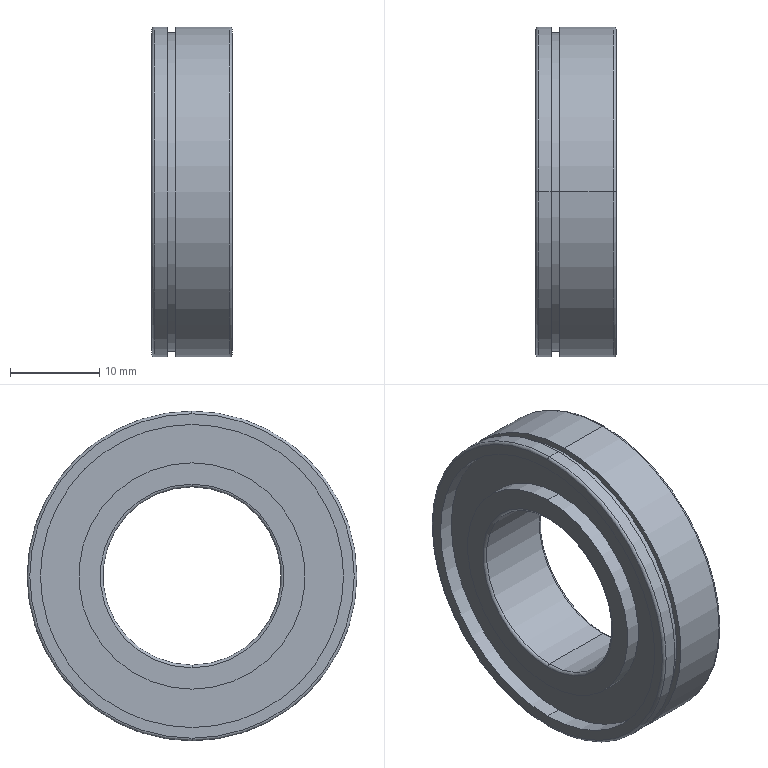Part | STEP file | SB6904ZZNR-Part-1-3 | 1 solid | 32 faces | box 9 x 37 x 37 mm | volume 5829 mm3 | cylinder 16 | torus 8 | plane 8 | commonest cylinder face diameters 25.4 x4 34 x4 37 x4 20 x2 35.7 x2
STEP:
#1=CARTESIAN_POINT('',(0.,0.,18.2));
#2=VERTEX_POINT('',#1);
#3=CARTESIAN_POINT('',(0.,0.,-18.2));
#4=VERTEX_POINT('',#3);
#5=CARTESIAN_POINT('',(0.,0.,0.));
#6=DIRECTION('',(-1.,0.,0.));
#7=DIRECTION('',(0.,0.,-1.));
#8=AXIS2_PLACEMENT_3D('',#5,#6,#7);
#9=CIRCLE('',#8,18.2);
#10=EDGE_CURVE('',#2,#4,#9,.T.);
#11=ORIENTED_EDGE('',*,*,#10,.F.);
#12=CARTESIAN_POINT('',(0.3,0.,18.5));
#13=VERTEX_POINT('',#12);
#14=CARTESIAN_POINT('',(0.3,0.,18.2));
#15=DIRECTION('',(0.,1.,0.));
#16=DIRECTION('',(0.,0.,1.));
#17=AXIS2_PLACEMENT_3D('',#14,#15,#16);
#18=CIRCLE('',#17,0.3);
#19=EDGE_CURVE('',#2,#13,#18,.T.);
#20=ORIENTED_EDGE('',*,*,#19,.T.);
#21=CARTESIAN_POINT('',(0.3,0.,-18.5));
#22=VERTEX_POINT('',#21);
#23=CARTESIAN_POINT('',(0.3,0.,0.));
#24=DIRECTION('',(1.,0.,0.));
#25=DIRECTION('',(0.,0.,-1.));
#26=AXIS2_PLACEMENT_3D('',#23,#24,#25);
#27=CIRCLE('',#26,18.5);
#28=EDGE_CURVE('',#22,#13,#27,.T.);
#29=ORIENTED_EDGE('',*,*,#28,.F.);
#30=CARTESIAN_POINT('',(0.3,0.,-18.2));
#31=DIRECTION('',(0.,-1.,0.));
#32=DIRECTION('',(0.,0.,-1.));
#33=AXIS2_PLACEMENT_3D('',#30,#31,#32);
#34=CIRCLE('',#33,0.3);
#35=EDGE_CURVE('',#4,#22,#34,.T.);
#36=ORIENTED_EDGE('',*,*,#35,.F.);
#37=EDGE_LOOP('',(#11,#20,#29,#36));
#38=FACE_OUTER_BOUND('',#37,.T.);
#39=CARTESIAN_POINT('',(0.3,0.,0.));
#40=DIRECTION('',(1.,0.,0.));
#41=DIRECTION('',(0.,0.,-1.));
#42=AXIS2_PLACEMENT_3D('',#39,#40,#41);
#43=TOROIDAL_SURFACE('',#42,18.2,0.3);
#44=ADVANCED_FACE('',(#38),#43,.T.);
#45=CARTESIAN_POINT('',(0.3,0.,10.));
#46=VERTEX_POINT('',#45);
#47=CARTESIAN_POINT('',(0.3,0.,-10.));
#48=VERTEX_POINT('',#47);
#49=CARTESIAN_POINT('',(0.3,0.,0.));
#50=DIRECTION('',(-1.,0.,0.));
#51=DIRECTION('',(0.,0.,-1.));
#52=AXIS2_PLACEMENT_3D('',#49,#50,#51);
#53=CIRCLE('',#52,10.);
#54=EDGE_CURVE('',#46,#48,#53,.T.);
#55=ORIENTED_EDGE('',*,*,#54,.F.);
#56=CARTESIAN_POINT('',(0.,0.,10.3));
#57=VERTEX_POINT('',#56);
#58=CARTESIAN_POINT('',(0.3,0.,10.3));
#59=DIRECTION('',(0.,1.,0.));
#60=DIRECTION('',(0.,0.,1.));
#61=AXIS2_PLACEMENT_3D('',#58,#59,#60);
#62=CIRCLE('',#61,0.3);
#63=EDGE_CURVE('',#46,#57,#62,.T.);
#64=ORIENTED_EDGE('',*,*,#63,.T.);
#65=CARTESIAN_POINT('',(0.,0.,-10.3));
#66=VERTEX_POINT('',#65);
#67=CARTESIAN_POINT('',(0.,0.,0.));
#68=DIRECTION('',(1.,0.,0.));
#69=DIRECTION('',(0.,0.,-1.));
#70=AXIS2_PLACEMENT_3D('',#67,#68,#69);
#71=CIRCLE('',#70,10.3);
#72=EDGE_CURVE('',#66,#57,#71,.T.);
#73=ORIENTED_EDGE('',*,*,#72,.F.);
#74=CARTESIAN_POINT('',(0.3,0.,-10.3));
#75=DIRECTION('',(0.,-1.,0.));
#76=DIRECTION('',(0.,0.,-1.));
#77=AXIS2_PLACEMENT_3D('',#74,#75,#76);
#78=CIRCLE('',#77,0.3);
#79=EDGE_CURVE('',#48,#66,#78,.T.);
#80=ORIENTED_EDGE('',*,*,#79,.F.);
#81=EDGE_LOOP('',(#55,#64,#73,#80));
#82=FACE_OUTER_BOUND('',#81,.T.);
#83=CARTESIAN_POINT('',(0.3,0.,0.));
#84=DIRECTION('',(1.,0.,0.));
#85=DIRECTION('',(0.,0.,-1.));
#86=AXIS2_PLACEMENT_3D('',#83,#84,#85);
#87=TOROIDAL_SURFACE('',#86,10.3,0.3);
#88=ADVANCED_FACE('',(#82),#87,.T.);
#89=CARTESIAN_POINT('',(8.7,0.,-10.));
#90=VERTEX_POINT('',#89);
#91=CARTESIAN_POINT('',(8.7,0.,10.));
#92=VERTEX_POINT('',#91);
#93=CARTESIAN_POINT('',(8.7,0.,0.));
#94=DIRECTION('',(1.,0.,0.));
#95=DIRECTION('',(0.,0.,1.));
#96=AXIS2_PLACEMENT_3D('',#93,#94,#95);
#97=CIRCLE('',#96,10.);
#98=EDGE_CURVE('',#90,#92,#97,.T.);
#99=ORIENTED_EDGE('',*,*,#98,.F.);
#100=CARTESIAN_POINT('',(9.,0.,-10.3));
#101=VERTEX_POINT('',#100);
#102=CARTESIAN_POINT('',(8.7,0.,-10.3));
#103=DIRECTION('',(0.,1.,0.));
#104=DIRECTION('',(0.,0.,1.));
#105=AXIS2_PLACEMENT_3D('',#102,#103,#104);
#106=CIRCLE('',#105,0.3);
#107=EDGE_CURVE('',#90,#101,#106,.T.);
#108=ORIENTED_EDGE('',*,*,#107,.T.);
#109=CARTESIAN_POINT('',(9.,0.,10.3));
#110=VERTEX_POINT('',#109);
#111=CARTESIAN_POINT('',(9.,0.,0.));
#112=DIRECTION('',(-1.,0.,0.));
#113=DIRECTION('',(0.,0.,1.));
#114=AXIS2_PLACEMENT_3D('',#111,#112,#113);
#115=CIRCLE('',#114,10.3);
#116=EDGE_CURVE('',#110,#101,#115,.T.);
#117=ORIENTED_EDGE('',*,*,#116,.F.);
#118=CARTESIAN_POINT('',(8.7,0.,10.3));
#119=DIRECTION('',(0.,-1.,0.));
#120=DIRECTION('',(0.,0.,-1.));
#121=AXIS2_PLACEMENT_3D('',#118,#119,#120);
#122=CIRCLE('',#121,0.3);
#123=EDGE_CURVE('',#92,#110,#122,.T.);
#124=ORIENTED_EDGE('',*,*,#123,.F.);
#125=EDGE_LOOP('',(#99,#108,#117,#124));
#126=FACE_OUTER_BOUND('',#125,.T.);
#127=CARTESIAN_POINT('',(8.7,0.,0.));
#128=DIRECTION('',(-1.,0.,0.));
#129=DIRECTION('',(0.,0.,1.));
#130=AXIS2_PLACEMENT_3D('',#127,#128,#129);
#131=TOROIDAL_SURFACE('',#130,10.3,0.3);
#132=ADVANCED_FACE('',(#126),#131,.T.);
#133=CARTESIAN_POINT('',(9.,0.,-18.2));
#134=VERTEX_POINT('',#133);
#135=CARTESIAN_POINT('',(9.,0.,18.2));
#136=VERTEX_POINT('',#135);
#137=CARTESIAN_POINT('',(9.,0.,0.));
#138=DIRECTION('',(1.,0.,0.));
#139=DIRECTION('',(0.,0.,1.));
#140=AXIS2_PLACEMENT_3D('',#137,#138,#139);
#141=CIRCLE('',#140,18.2);
#142=EDGE_CURVE('',#134,#136,#141,.T.);
#143=ORIENTED_EDGE('',*,*,#142,.F.);
#144=CARTESIAN_POINT('',(8.7,0.,-18.5));
#145=VERTEX_POINT('',#144);
#146=CARTESIAN_POINT('',(8.7,0.,-18.2));
#147=DIRECTION('',(0.,1.,0.));
#148=DIRECTION('',(0.,0.,1.));
#149=AXIS2_PLACEMENT_3D('',#146,#147,#148);
#150=CIRCLE('',#149,0.3);
#151=EDGE_CURVE('',#134,#145,#150,.T.);
#152=ORIENTED_EDGE('',*,*,#151,.T.);
#153=CARTESIAN_POINT('',(8.7,0.,18.5));
#154=VERTEX_POINT('',#153);
#155=CARTESIAN_POINT('',(8.7,0.,0.));
#156=DIRECTION('',(-1.,0.,0.));
#157=DIRECTION('',(0.,0.,1.));
#158=AXIS2_PLACEMENT_3D('',#155,#156,#157);
#159=CIRCLE('',#158,18.5);
#160=EDGE_CURVE('',#154,#145,#159,.T.);
#161=ORIENTED_EDGE('',*,*,#160,.F.);
#162=CARTESIAN_POINT('',(8.7,0.,18.2));
#163=DIRECTION('',(0.,-1.,0.));
#164=DIRECTION('',(0.,0.,-1.));
#165=AXIS2_PLACEMENT_3D('',#162,#163,#164);
#166=CIRCLE('',#165,0.3);
#167=EDGE_CURVE('',#136,#154,#166,.T.);
#168=ORIENTED_EDGE('',*,*,#167,.F.);
#169=EDGE_LOOP('',(#143,#152,#161,#168));
#170=FACE_OUTER_BOUND('',#169,.T.);
#171=CARTESIAN_POINT('',(8.7,0.,0.));
#172=DIRECTION('',(-1.,0.,0.));
#173=DIRECTION('',(0.,0.,1.));
#174=AXIS2_PLACEMENT_3D('',#171,#172,#173);
#175=TOROIDAL_SURFACE('',#174,18.2,0.3);
#176=ADVANCED_FACE('',(#170),#175,.T.);
#177=CARTESIAN_POINT('',(1.7,0.,-17.));
#178=VERTEX_POINT('',#177);
#179=CARTESIAN_POINT('',(1.7,0.,17.));
#180=VERTEX_POINT('',#179);
#181=CARTESIAN_POINT('',(1.7,0.,0.));
#182=DIRECTION('',(-1.,0.,0.));
#183=DIRECTION('',(0.,0.,1.));
#184=AXIS2_PLACEMENT_3D('',#181,#182,#183);
#185=CIRCLE('',#184,17.);
#186=EDGE_CURVE('',#178,#180,#185,.T.);
#187=ORIENTED_EDGE('',*,*,#186,.F.);
#188=CARTESIAN_POINT('',(0.,0.,-17.));
#189=VERTEX_POINT('',#188);
#190=CARTESIAN_POINT('',(0.,0.,-17.));
#191=DIRECTION('',(-1.,0.,0.));
#192=VECTOR('',#191,1000.);
#193=LINE('',#190,#192);
#194=EDGE_CURVE('',#178,#189,#193,.T.);
#195=ORIENTED_EDGE('',*,*,#194,.T.);
#196=CARTESIAN_POINT('',(0.,0.,17.));
#197=VERTEX_POINT('',#196);
#198=CARTESIAN_POINT('',(0.,0.,0.));
#199=DIRECTION('',(-1.,0.,0.));
#200=DIRECTION('',(0.,0.,1.));
#201=AXIS2_PLACEMENT_3D('',#198,#199,#200);
#202=CIRCLE('',#201,17.);
#203=EDGE_CURVE('',#189,#197,#202,.T.);
#204=ORIENTED_EDGE('',*,*,#203,.T.);
#205=CARTESIAN_POINT('',(0.,0.,17.));
#206=DIRECTION('',(-1.,0.,0.));
#207=VECTOR('',#206,1000.);
#208=LINE('',#205,#207);
#209=EDGE_CURVE('',#180,#197,#208,.T.);
#210=ORIENTED_EDGE('',*,*,#209,.F.);
#211=EDGE_LOOP('',(#187,#195,#204,#210));
#212=FACE_OUTER_BOUND('',#211,.T.);
#213=CARTESIAN_POINT('',(0.,0.,0.));
#214=DIRECTION('',(-1.,0.,0.));
#215=DIRECTION('',(0.,0.,1.));
#216=AXIS2_PLACEMENT_3D('',#213,#214,#215);
#217=CYLINDRICAL_SURFACE('',#216,17.);
#218=ADVANCED_FACE('',(#212),#217,.F.);
#219=CARTESIAN_POINT('',(1.7,0.,12.7));
#220=VERTEX_POINT('',#219);
#221=CARTESIAN_POINT('',(1.7,0.,-12.7));
#222=VERTEX_POINT('',#221);
#223=CARTESIAN_POINT('',(1.7,0.,0.));
#224=DIRECTION('',(-1.,0.,0.));
#225=DIRECTION('',(0.,0.,1.));
#226=AXIS2_PLACEMENT_3D('',#223,#224,#225);
#227=CIRCLE('',#226,12.7);
#228=EDGE_CURVE('',#220,#222,#227,.T.);
#229=ORIENTED_EDGE('',*,*,#228,.T.);
#230=CARTESIAN_POINT('',(0.,0.,-12.7));
#231=VERTEX_POINT('',#230);
#232=CARTESIAN_POINT('',(0.,0.,-12.7));
#233=DIRECTION('',(-1.,0.,0.));
#234=VECTOR('',#233,1000.);
#235=LINE('',#232,#234);
#236=EDGE_CURVE('',#222,#231,#235,.T.);
#237=ORIENTED_EDGE('',*,*,#236,.T.);
#238=CARTESIAN_POINT('',(0.,0.,12.7));
#239=VERTEX_POINT('',#238);
#240=CARTESIAN_POINT('',(0.,0.,0.));
#241=DIRECTION('',(-1.,0.,0.));
#242=DIRECTION('',(0.,0.,1.));
#243=AXIS2_PLACEMENT_3D('',#240,#241,#242);
#244=CIRCLE('',#243,12.7);
#245=EDGE_CURVE('',#239,#231,#244,.T.);
#246=ORIENTED_EDGE('',*,*,#245,.F.);
#247=CARTESIAN_POINT('',(0.,0.,12.7));
#248=DIRECTION('',(-1.,0.,0.));
#249=VECTOR('',#248,1000.);
#250=LINE('',#247,#249);
#251=EDGE_CURVE('',#220,#239,#250,.T.);
#252=ORIENTED_EDGE('',*,*,#251,.F.);
#253=EDGE_LOOP('',(#229,#237,#246,#252));
#254=FACE_OUTER_BOUND('',#253,.T.);
#255=CARTESIAN_POINT('',(0.,0.,0.));
#256=DIRECTION('',(-1.,0.,0.));
#257=DIRECTION('',(0.,0.,1.));
#258=AXIS2_PLACEMENT_3D('',#255,#256,#257);
#259=CYLINDRICAL_SURFACE('',#258,12.7);
#260=ADVANCED_FACE('',(#254),#259,.T.);
#261=CARTESIAN_POINT('',(8.7,0.,0.));
#262=DIRECTION('',(1.,0.,0.));
#263=DIRECTION('',(0.,0.,1.));
#264=AXIS2_PLACEMENT_3D('',#261,#262,#263);
#265=CIRCLE('',#264,10.);
#266=EDGE_CURVE('',#92,#90,#265,.T.);
#267=ORIENTED_EDGE('',*,*,#266,.T.);
#268=CARTESIAN_POINT('',(0.,0.,-10.));
#269=DIRECTION('',(-1.,0.,0.));
#270=VECTOR('',#269,1000.);
#271=LINE('',#268,#270);
#272=EDGE_CURVE('',#90,#48,#271,.T.);
#273=ORIENTED_EDGE('',*,*,#272,.T.);
#274=CARTESIAN_POINT('',(0.3,0.,0.));
#275=DIRECTION('',(-1.,0.,0.));
#276=DIRECTION('',(0.,0.,-1.));
#277=AXIS2_PLACEMENT_3D('',#274,#275,#276);
#278=CIRCLE('',#277,10.);
#279=EDGE_CURVE('',#48,#46,#278,.T.);
#280=ORIENTED_EDGE('',*,*,#279,.T.);
#281=CARTESIAN_POINT('',(0.,0.,10.));
#282=DIRECTION('',(-1.,0.,0.));
#283=VECTOR('',#282,1000.);
#284=LINE('',#281,#283);
#285=EDGE_CURVE('',#92,#46,#284,.T.);
#286=ORIENTED_EDGE('',*,*,#285,.F.);
#287=EDGE_LOOP('',(#267,#273,#280,#286));
#288=FACE_OUTER_BOUND('',#287,.T.);
#289=CARTESIAN_POINT('',(0.,0.,0.));
#290=DIRECTION('',(-1.,0.,0.));
#291=DIRECTION('',(0.,0.,1.));
#292=AXIS2_PLACEMENT_3D('',#289,#290,#291);
#293=CYLINDRICAL_SURFACE('',#292,10.);
#294=ADVANCED_FACE('',(#288),#293,.F.);
#295=CARTESIAN_POINT('',(9.,0.,12.7));
#296=VERTEX_POINT('',#295);
#297=CARTESIAN_POINT('',(9.,0.,-12.7));
#298=VERTEX_POINT('',#297);
#299=CARTESIAN_POINT('',(9.,0.,0.));
#300=DIRECTION('',(-1.,0.,0.));
#301=DIRECTION('',(0.,0.,1.));
#302=AXIS2_PLACEMENT_3D('',#299,#300,#301);
#303=CIRCLE('',#302,12.7);
#304=EDGE_CURVE('',#296,#298,#303,.T.);
#305=ORIENTED_EDGE('',*,*,#304,.T.);
#306=CARTESIAN_POINT('',(8.35,0.,-12.7));
#307=VERTEX_POINT('',#306);
#308=CARTESIAN_POINT('',(0.,0.,-12.7));
#309=DIRECTION('',(-1.,0.,0.));
#310=VECTOR('',#309,1000.);
#311=LINE('',#308,#310);
#312=EDGE_CURVE('',#298,#307,#311,.T.);
#313=ORIENTED_EDGE('',*,*,#312,.T.);
#314=CARTESIAN_POINT('',(8.35,0.,12.7));
#315=VERTEX_POINT('',#314);
#316=CARTESIAN_POINT('',(8.35,0.,0.));
#317=DIRECTION('',(-1.,0.,0.));
#318=DIRECTION('',(0.,0.,1.));
#319=AXIS2_PLACEMENT_3D('',#316,#317,#318);
#320=CIRCLE('',#319,12.7);
#321=EDGE_CURVE('',#315,#307,#320,.T.);
#322=ORIENTED_EDGE('',*,*,#321,.F.);
#323=CARTESIAN_POINT('',(0.,0.,12.7));
#324=DIRECTION('',(-1.,0.,0.));
#325=VECTOR('',#324,1000.);
#326=LINE('',#323,#325);
#327=EDGE_CURVE('',#296,#315,#326,.T.);
#328=ORIENTED_EDGE('',*,*,#327,.F.);
#329=EDGE_LOOP('',(#305,#313,#322,#328));
#330=FACE_OUTER_BOUND('',#329,.T.);
#331=CARTESIAN_POINT('',(0.,0.,0.));
#332=DIRECTION('',(-1.,0.,0.));
#333=DIRECTION('',(0.,0.,1.));
#334=AXIS2_PLACEMENT_3D('',#331,#332,#333);
#335=CYLINDRICAL_SURFACE('',#334,12.7);
#336=ADVANCED_FACE('',(#330),#335,.T.);
#337=CARTESIAN_POINT('',(9.,0.,-17.));
#338=VERTEX_POINT('',#337);
#339=CARTESIAN_POINT('',(9.,0.,17.));
#340=VERTEX_POINT('',#339);
#341=CARTESIAN_POINT('',(9.,0.,0.));
#342=DIRECTION('',(-1.,0.,0.));
#343=DIRECTION('',(0.,0.,1.));
#344=AXIS2_PLACEMENT_3D('',#341,#342,#343);
#345=CIRCLE('',#344,17.);
#346=EDGE_CURVE('',#338,#340,#345,.T.);
#347=ORIENTED_EDGE('',*,*,#346,.F.);
#348=CARTESIAN_POINT('',(8.35,0.,-17.));
#349=VERTEX_POINT('',#348);
#350=CARTESIAN_POINT('',(0.,0.,-17.));
#351=DIRECTION('',(-1.,0.,0.));
#352=VECTOR('',#351,1000.);
#353=LINE('',#350,#352);
#354=EDGE_CURVE('',#338,#349,#353,.T.);
#355=ORIENTED_EDGE('',*,*,#354,.T.);
#356=CARTESIAN_POINT('',(8.35,0.,17.));
#357=VERTEX_POINT('',#356);
#358=CARTESIAN_POINT('',(8.35,0.,0.));
#359=DIRECTION('',(-1.,0.,0.));
#360=DIRECTION('',(0.,0.,1.));
#361=AXIS2_PLACEMENT_3D('',#358,#359,#360);
#362=CIRCLE('',#361,17.);
#363=EDGE_CURVE('',#349,#357,#362,.T.);
#364=ORIENTED_EDGE('',*,*,#363,.T.);
#365=CARTESIAN_POINT('',(0.,0.,17.));
#366=DIRECTION('',(-1.,0.,0.));
#367=VECTOR('',#366,1000.);
#368=LINE('',#365,#367);
#369=EDGE_CURVE('',#340,#357,#368,.T.);
#370=ORIENTED_EDGE('',*,*,#369,.F.);
#371=EDGE_LOOP('',(#347,#355,#364,#370));
#372=FACE_OUTER_BOUND('',#371,.T.);
#373=CARTESIAN_POINT('',(0.,0.,0.));
#374=DIRECTION('',(-1.,0.,0.));
#375=DIRECTION('',(0.,0.,1.));
#376=AXIS2_PLACEMENT_3D('',#373,#374,#375);
#377=CYLINDRICAL_SURFACE('',#376,17.);
#378=ADVANCED_FACE('',(#372),#377,.F.);
#379=ORIENTED_EDGE('',*,*,#160,.T.);
#380=CARTESIAN_POINT('',(2.65,0.,-18.5));
#381=VERTEX_POINT('',#380);
#382=CARTESIAN_POINT('',(0.,0.,-18.5));
#383=DIRECTION('',(-1.,0.,0.));
#384=VECTOR('',#383,1000.);
#385=LINE('',#382,#384);
#386=EDGE_CURVE('',#145,#381,#385,.T.);
#387=ORIENTED_EDGE('',*,*,#386,.T.);
#388=CARTESIAN_POINT('',(2.65,0.,18.5));
#389=VERTEX_POINT('',#388);
#390=CARTESIAN_POINT('',(2.65,0.,0.));
#391=DIRECTION('',(-1.,0.,0.));
#392=DIRECTION('',(0.,0.,1.));
#393=AXIS2_PLACEMENT_3D('',#390,#391,#392);
#394=CIRCLE('',#393,18.5);
#395=EDGE_CURVE('',#389,#381,#394,.T.);
#396=ORIENTED_EDGE('',*,*,#395,.F.);
#397=CARTESIAN_POINT('',(0.,0.,18.5));
#398=DIRECTION('',(-1.,0.,0.));
#399=VECTOR('',#398,1000.);
#400=LINE('',#397,#399);
#401=EDGE_CURVE('',#154,#389,#400,.T.);
#402=ORIENTED_EDGE('',*,*,#401,.F.);
#403=EDGE_LOOP('',(#379,#387,#396,#402));
#404=FACE_OUTER_BOUND('',#403,.T.);
#405=CARTESIAN_POINT('',(0.,0.,0.));
#406=DIRECTION('',(-1.,0.,0.));
#407=DIRECTION('',(0.,0.,1.));
#408=AXIS2_PLACEMENT_3D('',#405,#406,#407);
#409=CYLINDRICAL_SURFACE('',#408,18.5);
#410=ADVANCED_FACE('',(#404),#409,.T.);
#411=CARTESIAN_POINT('',(2.65,0.,17.85));
#412=VERTEX_POINT('',#411);
#413=CARTESIAN_POINT('',(2.65,0.,-17.85));
#414=VERTEX_POINT('',#413);
#415=CARTESIAN_POINT('',(2.65,0.,0.));
#416=DIRECTION('',(-1.,0.,0.));
#417=DIRECTION('',(0.,0.,1.));
#418=AXIS2_PLACEMENT_3D('',#415,#416,#417);
#419=CIRCLE('',#418,17.85);
#420=EDGE_CURVE('',#412,#414,#419,.T.);
#421=ORIENTED_EDGE('',*,*,#420,.T.);
#422=CARTESIAN_POINT('',(1.7,0.,-17.85));
#423=VERTEX_POINT('',#422);
#424=CARTESIAN_POINT('',(1.05,0.,-17.85));
#425=DIRECTION('',(-1.,0.,0.));
#426=VECTOR('',#425,1000.);
#427=LINE('',#424,#426);
#428=EDGE_CURVE('',#414,#423,#427,.T.);
#429=ORIENTED_EDGE('',*,*,#428,.T.);
#430=CARTESIAN_POINT('',(1.7,0.,17.85));
#431=VERTEX_POINT('',#430);
#432=CARTESIAN_POINT('',(1.7,0.,0.));
#433=DIRECTION('',(-1.,0.,0.));
#434=DIRECTION('',(0.,0.,1.));
#435=AXIS2_PLACEMENT_3D('',#432,#433,#434);
#436=CIRCLE('',#435,17.85);
#437=EDGE_CURVE('',#431,#423,#436,.T.);
#438=ORIENTED_EDGE('',*,*,#437,.F.);
#439=CARTESIAN_POINT('',(1.05,0.,17.85));
#440=DIRECTION('',(-1.,0.,0.));
#441=VECTOR('',#440,1000.);
#442=LINE('',#439,#441);
#443=EDGE_CURVE('',#412,#431,#442,.T.);
#444=ORIENTED_EDGE('',*,*,#443,.F.);
#445=EDGE_LOOP('',(#421,#429,#438,#444));
#446=FACE_OUTER_BOUND('',#445,.T.);
#447=CARTESIAN_POINT('',(1.05,0.,0.));
#448=DIRECTION('',(-1.,0.,0.));
#449=DIRECTION('',(0.,0.,1.));
#450=AXIS2_PLACEMENT_3D('',#447,#448,#449);
#451=CYLINDRICAL_SURFACE('',#450,17.85);
#452=ADVANCED_FACE('',(#446),#451,.T.);
#453=CARTESIAN_POINT('',(1.7,0.,18.5));
#454=VERTEX_POINT('',#453);
#455=CARTESIAN_POINT('',(1.7,0.,-18.5));
#456=VERTEX_POINT('',#455);
#457=CARTESIAN_POINT('',(1.7,0.,0.));
#458=DIRECTION('',(-1.,0.,0.));
#459=DIRECTION('',(0.,0.,1.));
#460=AXIS2_PLACEMENT_3D('',#457,#458,#459);
#461=CIRCLE('',#460,18.5);
#462=EDGE_CURVE('',#454,#456,#461,.T.);
#463=ORIENTED_EDGE('',*,*,#462,.T.);
#464=CARTESIAN_POINT('',(0.,0.,-18.5));
#465=DIRECTION('',(-1.,0.,0.));
#466=VECTOR('',#465,1000.);
#467=LINE('',#464,#466);
#468=EDGE_CURVE('',#456,#22,#467,.T.);
#469=ORIENTED_EDGE('',*,*,#468,.T.);
#470=ORIENTED_EDGE('',*,*,#28,.T.);
#471=CARTESIAN_POINT('',(0.,0.,18.5));
#472=DIRECTION('',(-1.,0.,0.));
#473=VECTOR('',#472,1000.);
#474=LINE('',#471,#473);
#475=EDGE_CURVE('',#454,#13,#474,.T.);
#476=ORIENTED_EDGE('',*,*,#475,.F.);
#477=EDGE_LOOP('',(#463,#469,#470,#476));
#478=FACE_OUTER_BOUND('',#477,.T.);
#479=CARTESIAN_POINT('',(0.,0.,0.));
#480=DIRECTION('',(-1.,0.,0.));
#481=DIRECTION('',(0.,0.,1.));
#482=AXIS2_PLACEMENT_3D('',#479,#480,#481);
#483=CYLINDRICAL_SURFACE('',#482,18.5);
#484=ADVANCED_FACE('',(#478),#483,.T.);
#485=CARTESIAN_POINT('',(0.,0.,0.));
#486=DIRECTION('',(-1.,0.,0.));
#487=DIRECTION('',(0.,0.,-1.));
#488=AXIS2_PLACEMENT_3D('',#485,#486,#487);
#489=CIRCLE('',#488,18.2);
#490=EDGE_CURVE('',#4,#2,#489,.T.);
#491=ORIENTED_EDGE('',*,*,#490,.T.);
#492=ORIENTED_EDGE('',*,*,#10,.T.);
#493=EDGE_LOOP('',(#491,#492));
#494=FACE_OUTER_BOUND('',#493,.T.);
#495=CARTESIAN_POINT('',(0.,0.,0.));
#496=DIRECTION('',(-1.,0.,0.));
#497=DIRECTION('',(0.,0.,1.));
#498=AXIS2_PLACEMENT_3D('',#495,#496,#497);
#499=CIRCLE('',#498,17.);
#500=EDGE_CURVE('',#197,#189,#499,.T.);
#501=ORIENTED_EDGE('',*,*,#500,.F.);
#502=ORIENTED_EDGE('',*,*,#203,.F.);
#503=EDGE_LOOP('',(#501,#502));
#504=FACE_BOUND('',#503,.T.);
#505=CARTESIAN_POINT('',(0.,17.,0.));
#506=DIRECTION('',(1.,0.,0.));
#507=DIRECTION('',(0.,0.,-1.));
#508=AXIS2_PLACEMENT_3D('',#505,#506,#507);
#509=PLANE('',#508);
#510=ADVANCED_FACE('',(#494,#504),#509,.F.);
#511=ORIENTED_EDGE('',*,*,#468,.F.);
#512=CARTESIAN_POINT('',(1.7,0.,0.));
#513=DIRECTION('',(-1.,0.,0.));
#514=DIRECTION('',(0.,0.,1.));
#515=AXIS2_PLACEMENT_3D('',#512,#513,#514);
#516=CIRCLE('',#515,18.5);
#517=EDGE_CURVE('',#456,#454,#516,.T.);
#518=ORIENTED_EDGE('',*,*,#517,.T.);
#519=ORIENTED_EDGE('',*,*,#475,.T.);
#520=CARTESIAN_POINT('',(0.3,0.,0.));
#521=DIRECTION('',(1.,0.,0.));
#522=DIRECTION('',(0.,0.,-1.));
#523=AXIS2_PLACEMENT_3D('',#520,#521,#522);
#524=CIRCLE('',#523,18.5);
#525=EDGE_CURVE('',#13,#22,#524,.T.);
#526=ORIENTED_EDGE('',*,*,#525,.T.);
#527=EDGE_LOOP('',(#511,#518,#519,#526));
#528=FACE_OUTER_BOUND('',#527,.T.);
#529=CARTESIAN_POINT('',(0.,0.,0.));
#530=DIRECTION('',(-1.,0.,0.));
#531=DIRECTION('',(0.,0.,1.));
#532=AXIS2_PLACEMENT_3D('',#529,#530,#531);
#533=CYLINDRICAL_SURFACE('',#532,18.5);
#534=ADVANCED_FACE('',(#528),#533,.T.);
#535=ORIENTED_EDGE('',*,*,#462,.F.);
#536=ORIENTED_EDGE('',*,*,#517,.F.);
#537=EDGE_LOOP('',(#535,#536));
#538=FACE_OUTER_BOUND('',#537,.T.);
#539=ORIENTED_EDGE('',*,*,#437,.T.);
#540=CARTESIAN_POINT('',(1.7,0.,0.));
#541=DIRECTION('',(-1.,0.,0.));
#542=DIRECTION('',(0.,0.,1.));
#543=AXIS2_PLACEMENT_3D('',#540,#541,#542);
#544=CIRCLE('',#543,17.85);
#545=EDGE_CURVE('',#423,#431,#544,.T.);
#546=ORIENTED_EDGE('',*,*,#545,.T.);
#547=EDGE_LOOP('',(#539,#546));
#548=FACE_BOUND('',#547,.T.);
#549=CARTESIAN_POINT('',(1.7,18.5,0.));
#550=DIRECTION('',(-1.,0.,0.));
#551=DIRECTION('',(0.,0.,1.));
#552=AXIS2_PLACEMENT_3D('',#549,#550,#551);
#553=PLANE('',#552);
#554=ADVANCED_FACE('',(#538,#548),#553,.F.);
#555=ORIENTED_EDGE('',*,*,#428,.F.);
#556=CARTESIAN_POINT('',(2.65,0.,0.));
#557=DIRECTION('',(-1.,0.,0.));
#558=DIRECTION('',(0.,0.,1.));
#559=AXIS2_PLACEMENT_3D('',#556,#557,#558);
#560=CIRCLE('',#559,17.85);
#561=EDGE_CURVE('',#414,#412,#560,.T.);
#562=ORIENTED_EDGE('',*,*,#561,.T.);
#563=ORIENTED_EDGE('',*,*,#443,.T.);
#564=ORIENTED_EDGE('',*,*,#545,.F.);
#565=EDGE_LOOP('',(#555,#562,#563,#564));
#566=FACE_OUTER_BOUND('',#565,.T.);
#567=CARTESIAN_POINT('',(1.05,0.,0.));
#568=DIRECTION('',(-1.,0.,0.));
#569=DIRECTION('',(0.,0.,1.));
#570=AXIS2_PLACEMENT_3D('',#567,#568,#569);
#571=CYLINDRICAL_SURFACE('',#570,17.85);
#572=ADVANCED_FACE('',(#566),#571,.T.);
#573=ORIENTED_EDGE('',*,*,#420,.F.);
#574=ORIENTED_EDGE('',*,*,#561,.F.);
#575=EDGE_LOOP('',(#573,#574));
#576=FACE_BOUND('',#575,.T.);
#577=ORIENTED_EDGE('',*,*,#395,.T.);
#578=CARTESIAN_POINT('',(2.65,0.,0.));
#579=DIRECTION('',(-1.,0.,0.));
#580=DIRECTION('',(0.,0.,1.));
#581=AXIS2_PLACEMENT_3D('',#578,#579,#580);
#582=CIRCLE('',#581,18.5);
#583=EDGE_CURVE('',#381,#389,#582,.T.);
#584=ORIENTED_EDGE('',*,*,#583,.T.);
#585=EDGE_LOOP('',(#577,#584));
#586=FACE_OUTER_BOUND('',#585,.T.);
#587=CARTESIAN_POINT('',(2.65,17.85,0.));
#588=DIRECTION('',(1.,0.,0.));
#589=DIRECTION('',(0.,0.,-1.));
#590=AXIS2_PLACEMENT_3D('',#587,#588,#589);
#591=PLANE('',#590);
#592=ADVANCED_FACE('',(#576,#586),#591,.F.);
#593=ORIENTED_EDGE('',*,*,#386,.F.);
#594=CARTESIAN_POINT('',(8.7,0.,0.));
#595=DIRECTION('',(-1.,0.,0.));
#596=DIRECTION('',(0.,0.,1.));
#597=AXIS2_PLACEMENT_3D('',#594,#595,#596);
#598=CIRCLE('',#597,18.5);
#599=EDGE_CURVE('',#145,#154,#598,.T.);
#600=ORIENTED_EDGE('',*,*,#599,.T.);
#601=ORIENTED_EDGE('',*,*,#401,.T.);
#602=ORIENTED_EDGE('',*,*,#583,.F.);
#603=EDGE_LOOP('',(#593,#600,#601,#602));
#604=FACE_OUTER_BOUND('',#603,.T.);
#605=CARTESIAN_POINT('',(0.,0.,0.));
#606=DIRECTION('',(-1.,0.,0.));
#607=DIRECTION('',(0.,0.,1.));
#608=AXIS2_PLACEMENT_3D('',#605,#606,#607);
#609=CYLINDRICAL_SURFACE('',#608,18.5);
#610=ADVANCED_FACE('',(#604),#609,.T.);
#611=CARTESIAN_POINT('',(9.,0.,0.));
#612=DIRECTION('',(1.,0.,0.));
#613=DIRECTION('',(0.,0.,1.));
#614=AXIS2_PLACEMENT_3D('',#611,#612,#613);
#615=CIRCLE('',#614,18.2);
#616=EDGE_CURVE('',#136,#134,#615,.T.);
#617=ORIENTED_EDGE('',*,*,#616,.T.);
#618=ORIENTED_EDGE('',*,*,#142,.T.);
#619=EDGE_LOOP('',(#617,#618));
#620=FACE_OUTER_BOUND('',#619,.T.);
#621=CARTESIAN_POINT('',(9.,0.,0.));
#622=DIRECTION('',(-1.,0.,0.));
#623=DIRECTION('',(0.,0.,1.));
#624=AXIS2_PLACEMENT_3D('',#621,#622,#623);
#625=CIRCLE('',#624,17.);
#626=EDGE_CURVE('',#340,#338,#625,.T.);
#627=ORIENTED_EDGE('',*,*,#626,.T.);
#628=ORIENTED_EDGE('',*,*,#346,.T.);
#629=EDGE_LOOP('',(#627,#628));
#630=FACE_BOUND('',#629,.T.);
#631=CARTESIAN_POINT('',(9.,18.5,0.));
#632=DIRECTION('',(-1.,0.,0.));
#633=DIRECTION('',(0.,0.,1.));
#634=AXIS2_PLACEMENT_3D('',#631,#632,#633);
#635=PLANE('',#634);
#636=ADVANCED_FACE('',(#620,#630),#635,.F.);
#637=ORIENTED_EDGE('',*,*,#354,.F.);
#638=ORIENTED_EDGE('',*,*,#626,.F.);
#639=ORIENTED_EDGE('',*,*,#369,.T.);
#640=CARTESIAN_POINT('',(8.35,0.,0.));
#641=DIRECTION('',(-1.,0.,0.));
#642=DIRECTION('',(0.,0.,1.));
#643=AXIS2_PLACEMENT_3D('',#640,#641,#642);
#644=CIRCLE('',#643,17.);
#645=EDGE_CURVE('',#357,#349,#644,.T.);
#646=ORIENTED_EDGE('',*,*,#645,.T.);
#647=EDGE_LOOP('',(#637,#638,#639,#646));
#648=FACE_OUTER_BOUND('',#647,.T.);
#649=CARTESIAN_POINT('',(0.,0.,0.));
#650=DIRECTION('',(-1.,0.,0.));
#651=DIRECTION('',(0.,0.,1.));
#652=AXIS2_PLACEMENT_3D('',#649,#650,#651);
#653=CYLINDRICAL_SURFACE('',#652,17.);
#654=ADVANCED_FACE('',(#648),#653,.F.);
#655=ORIENTED_EDGE('',*,*,#645,.F.);
#656=ORIENTED_EDGE('',*,*,#363,.F.);
#657=EDGE_LOOP('',(#655,#656));
#658=FACE_OUTER_BOUND('',#657,.T.);
#659=ORIENTED_EDGE('',*,*,#321,.T.);
#660=CARTESIAN_POINT('',(8.35,0.,0.));
#661=DIRECTION('',(-1.,0.,0.));
#662=DIRECTION('',(0.,0.,1.));
#663=AXIS2_PLACEMENT_3D('',#660,#661,#662);
#664=CIRCLE('',#663,12.7);
#665=EDGE_CURVE('',#307,#315,#664,.T.);
#666=ORIENTED_EDGE('',*,*,#665,.T.);
#667=EDGE_LOOP('',(#659,#666));
#668=FACE_BOUND('',#667,.T.);
#669=CARTESIAN_POINT('',(8.35,17.,0.));
#670=DIRECTION('',(-1.,0.,0.));
#671=DIRECTION('',(0.,0.,1.));
#672=AXIS2_PLACEMENT_3D('',#669,#670,#671);
#673=PLANE('',#672);
#674=ADVANCED_FACE('',(#658,#668),#673,.F.);
#675=ORIENTED_EDGE('',*,*,#312,.F.);
#676=CARTESIAN_POINT('',(9.,0.,0.));
#677=DIRECTION('',(-1.,0.,0.));
#678=DIRECTION('',(0.,0.,1.));
#679=AXIS2_PLACEMENT_3D('',#676,#677,#678);
#680=CIRCLE('',#679,12.7);
#681=EDGE_CURVE('',#298,#296,#680,.T.);
#682=ORIENTED_EDGE('',*,*,#681,.T.);
#683=ORIENTED_EDGE('',*,*,#327,.T.);
#684=ORIENTED_EDGE('',*,*,#665,.F.);
#685=EDGE_LOOP('',(#675,#682,#683,#684));
#686=FACE_OUTER_BOUND('',#685,.T.);
#687=CARTESIAN_POINT('',(0.,0.,0.));
#688=DIRECTION('',(-1.,0.,0.));
#689=DIRECTION('',(0.,0.,1.));
#690=AXIS2_PLACEMENT_3D('',#687,#688,#689);
#691=CYLINDRICAL_SURFACE('',#690,12.7);
#692=ADVANCED_FACE('',(#686),#691,.T.);
#693=ORIENTED_EDGE('',*,*,#116,.T.);
#694=CARTESIAN_POINT('',(9.,0.,0.));
#695=DIRECTION('',(-1.,0.,0.));
#696=DIRECTION('',(0.,0.,1.));
#697=AXIS2_PLACEMENT_3D('',#694,#695,#696);
#698=CIRCLE('',#697,10.3);
#699=EDGE_CURVE('',#101,#110,#698,.T.);
#700=ORIENTED_EDGE('',*,*,#699,.T.);
#701=EDGE_LOOP('',(#693,#700));
#702=FACE_BOUND('',#701,.T.);
#703=ORIENTED_EDGE('',*,*,#304,.F.);
#704=ORIENTED_EDGE('',*,*,#681,.F.);
#705=EDGE_LOOP('',(#703,#704));
#706=FACE_OUTER_BOUND('',#705,.T.);
#707=CARTESIAN_POINT('',(9.,12.7,0.));
#708=DIRECTION('',(-1.,0.,0.));
#709=DIRECTION('',(0.,0.,1.));
#710=AXIS2_PLACEMENT_3D('',#707,#708,#709);
#711=PLANE('',#710);
#712=ADVANCED_FACE('',(#702,#706),#711,.F.);
#713=ORIENTED_EDGE('',*,*,#272,.F.);
#714=ORIENTED_EDGE('',*,*,#98,.T.);
#715=ORIENTED_EDGE('',*,*,#285,.T.);
#716=ORIENTED_EDGE('',*,*,#54,.T.);
#717=EDGE_LOOP('',(#713,#714,#715,#716));
#718=FACE_OUTER_BOUND('',#717,.T.);
#719=CARTESIAN_POINT('',(0.,0.,0.));
#720=DIRECTION('',(-1.,0.,0.));
#721=DIRECTION('',(0.,0.,1.));
#722=AXIS2_PLACEMENT_3D('',#719,#720,#721);
#723=CYLINDRICAL_SURFACE('',#722,10.);
#724=ADVANCED_FACE('',(#718),#723,.F.);
#725=ORIENTED_EDGE('',*,*,#72,.T.);
#726=CARTESIAN_POINT('',(0.,0.,0.));
#727=DIRECTION('',(1.,0.,0.));
#728=DIRECTION('',(0.,0.,-1.));
#729=AXIS2_PLACEMENT_3D('',#726,#727,#728);
#730=CIRCLE('',#729,10.3);
#731=EDGE_CURVE('',#57,#66,#730,.T.);
#732=ORIENTED_EDGE('',*,*,#731,.T.);
#733=EDGE_LOOP('',(#725,#732));
#734=FACE_BOUND('',#733,.T.);
#735=ORIENTED_EDGE('',*,*,#245,.T.);
#736=CARTESIAN_POINT('',(0.,0.,0.));
#737=DIRECTION('',(-1.,0.,0.));
#738=DIRECTION('',(0.,0.,1.));
#739=AXIS2_PLACEMENT_3D('',#736,#737,#738);
#740=CIRCLE('',#739,12.7);
#741=EDGE_CURVE('',#231,#239,#740,.T.);
#742=ORIENTED_EDGE('',*,*,#741,.T.);
#743=EDGE_LOOP('',(#735,#742));
#744=FACE_OUTER_BOUND('',#743,.T.);
#745=CARTESIAN_POINT('',(0.,10.,0.));
#746=DIRECTION('',(1.,0.,0.));
#747=DIRECTION('',(0.,0.,-1.));
#748=AXIS2_PLACEMENT_3D('',#745,#746,#747);
#749=PLANE('',#748);
#750=ADVANCED_FACE('',(#734,#744),#749,.F.);
#751=ORIENTED_EDGE('',*,*,#236,.F.);
#752=CARTESIAN_POINT('',(1.7,0.,0.));
#753=DIRECTION('',(-1.,0.,0.));
#754=DIRECTION('',(0.,0.,1.));
#755=AXIS2_PLACEMENT_3D('',#752,#753,#754);
#756=CIRCLE('',#755,12.7);
#757=EDGE_CURVE('',#222,#220,#756,.T.);
#758=ORIENTED_EDGE('',*,*,#757,.T.);
#759=ORIENTED_EDGE('',*,*,#251,.T.);
#760=ORIENTED_EDGE('',*,*,#741,.F.);
#761=EDGE_LOOP('',(#751,#758,#759,#760));
#762=FACE_OUTER_BOUND('',#761,.T.);
#763=CARTESIAN_POINT('',(0.,0.,0.));
#764=DIRECTION('',(-1.,0.,0.));
#765=DIRECTION('',(0.,0.,1.));
#766=AXIS2_PLACEMENT_3D('',#763,#764,#765);
#767=CYLINDRICAL_SURFACE('',#766,12.7);
#768=ADVANCED_FACE('',(#762),#767,.T.);
#769=ORIENTED_EDGE('',*,*,#228,.F.);
#770=ORIENTED_EDGE('',*,*,#757,.F.);
#771=EDGE_LOOP('',(#769,#770));
#772=FACE_BOUND('',#771,.T.);
#773=CARTESIAN_POINT('',(1.7,0.,0.));
#774=DIRECTION('',(-1.,0.,0.));
#775=DIRECTION('',(0.,0.,1.));
#776=AXIS2_PLACEMENT_3D('',#773,#774,#775);
#777=CIRCLE('',#776,17.);
#778=EDGE_CURVE('',#180,#178,#777,.T.);
#779=ORIENTED_EDGE('',*,*,#778,.T.);
#780=ORIENTED_EDGE('',*,*,#186,.T.);
#781=EDGE_LOOP('',(#779,#780));
#782=FACE_OUTER_BOUND('',#781,.T.);
#783=CARTESIAN_POINT('',(1.7,17.,0.));
#784=DIRECTION('',(1.,0.,0.));
#785=DIRECTION('',(0.,0.,-1.));
#786=AXIS2_PLACEMENT_3D('',#783,#784,#785);
#787=PLANE('',#786);
#788=ADVANCED_FACE('',(#772,#782),#787,.F.);
#789=ORIENTED_EDGE('',*,*,#194,.F.);
#790=ORIENTED_EDGE('',*,*,#778,.F.);
#791=ORIENTED_EDGE('',*,*,#209,.T.);
#792=ORIENTED_EDGE('',*,*,#500,.T.);
#793=EDGE_LOOP('',(#789,#790,#791,#792));
#794=FACE_OUTER_BOUND('',#793,.T.);
#795=CARTESIAN_POINT('',(0.,0.,0.));
#796=DIRECTION('',(-1.,0.,0.));
#797=DIRECTION('',(0.,0.,1.));
#798=AXIS2_PLACEMENT_3D('',#795,#796,#797);
#799=CYLINDRICAL_SURFACE('',#798,17.);
#800=ADVANCED_FACE('',(#794),#799,.F.);
#801=ORIENTED_EDGE('',*,*,#151,.F.);
#802=ORIENTED_EDGE('',*,*,#616,.F.);
#803=ORIENTED_EDGE('',*,*,#167,.T.);
#804=ORIENTED_EDGE('',*,*,#599,.F.);
#805=EDGE_LOOP('',(#801,#802,#803,#804));
#806=FACE_OUTER_BOUND('',#805,.T.);
#807=CARTESIAN_POINT('',(8.7,0.,0.));
#808=DIRECTION('',(-1.,0.,0.));
#809=DIRECTION('',(0.,0.,1.));
#810=AXIS2_PLACEMENT_3D('',#807,#808,#809);
#811=TOROIDAL_SURFACE('',#810,18.2,0.3);
#812=ADVANCED_FACE('',(#806),#811,.T.);
#813=ORIENTED_EDGE('',*,*,#107,.F.);
#814=ORIENTED_EDGE('',*,*,#266,.F.);
#815=ORIENTED_EDGE('',*,*,#123,.T.);
#816=ORIENTED_EDGE('',*,*,#699,.F.);
#817=EDGE_LOOP('',(#813,#814,#815,#816));
#818=FACE_OUTER_BOUND('',#817,.T.);
#819=CARTESIAN_POINT('',(8.7,0.,0.));
#820=DIRECTION('',(-1.,0.,0.));
#821=DIRECTION('',(0.,0.,1.));
#822=AXIS2_PLACEMENT_3D('',#819,#820,#821);
#823=TOROIDAL_SURFACE('',#822,10.3,0.3);
#824=ADVANCED_FACE('',(#818),#823,.T.);
#825=ORIENTED_EDGE('',*,*,#63,.F.);
#826=ORIENTED_EDGE('',*,*,#279,.F.);
#827=ORIENTED_EDGE('',*,*,#79,.T.);
#828=ORIENTED_EDGE('',*,*,#731,.F.);
#829=EDGE_LOOP('',(#825,#826,#827,#828));
#830=FACE_OUTER_BOUND('',#829,.T.);
#831=CARTESIAN_POINT('',(0.3,0.,0.));
#832=DIRECTION('',(1.,0.,0.));
#833=DIRECTION('',(0.,0.,-1.));
#834=AXIS2_PLACEMENT_3D('',#831,#832,#833);
#835=TOROIDAL_SURFACE('',#834,10.3,0.3);
#836=ADVANCED_FACE('',(#830),#835,.T.);
#837=ORIENTED_EDGE('',*,*,#19,.F.);
#838=ORIENTED_EDGE('',*,*,#490,.F.);
#839=ORIENTED_EDGE('',*,*,#35,.T.);
#840=ORIENTED_EDGE('',*,*,#525,.F.);
#841=EDGE_LOOP('',(#837,#838,#839,#840));
#842=FACE_OUTER_BOUND('',#841,.T.);
#843=CARTESIAN_POINT('',(0.3,0.,0.));
#844=DIRECTION('',(1.,0.,0.));
#845=DIRECTION('',(0.,0.,-1.));
#846=AXIS2_PLACEMENT_3D('',#843,#844,#845);
#847=TOROIDAL_SURFACE('',#846,18.2,0.3);
#848=ADVANCED_FACE('',(#842),#847,.T.);
#849=CLOSED_SHELL('',(#44,#88,#132,#176,#218,#260,#294,#336,#378,#410,#452,#484,#510,#534,#554,#572,#592,#610,#636,#654,#674,#692,#712,#724,#750,#768,#788,#800,#812,#824,#836,#848));
#850=MANIFOLD_SOLID_BREP('',#849);
#851=CARTESIAN_POINT('',(0.,0.,0.));
#852=DIRECTION('',(0.,0.,1.));
#853=DIRECTION('',(1.,0.,0.));
#854=AXIS2_PLACEMENT_3D('',#851,#852,#853);
#855=(LENGTH_UNIT()NAMED_UNIT(*)SI_UNIT(.MILLI.,.METRE.));
#856=UNCERTAINTY_MEASURE_WITH_UNIT(LENGTH_MEASURE(0.00001),#855,'','');
#857=(NAMED_UNIT(*)PLANE_ANGLE_UNIT()SI_UNIT($,.RADIAN.));
#858=(NAMED_UNIT(*)SI_UNIT($,.STERADIAN.)SOLID_ANGLE_UNIT());
#859=(GEOMETRIC_REPRESENTATION_CONTEXT(3)GLOBAL_UNCERTAINTY_ASSIGNED_CONTEXT((#856))GLOBAL_UNIT_ASSIGNED_CONTEXT((#855,#857,#858))REPRESENTATION_CONTEXT('',''));
#860=ADVANCED_BREP_SHAPE_REPRESENTATION('',(#850,#854),#859);